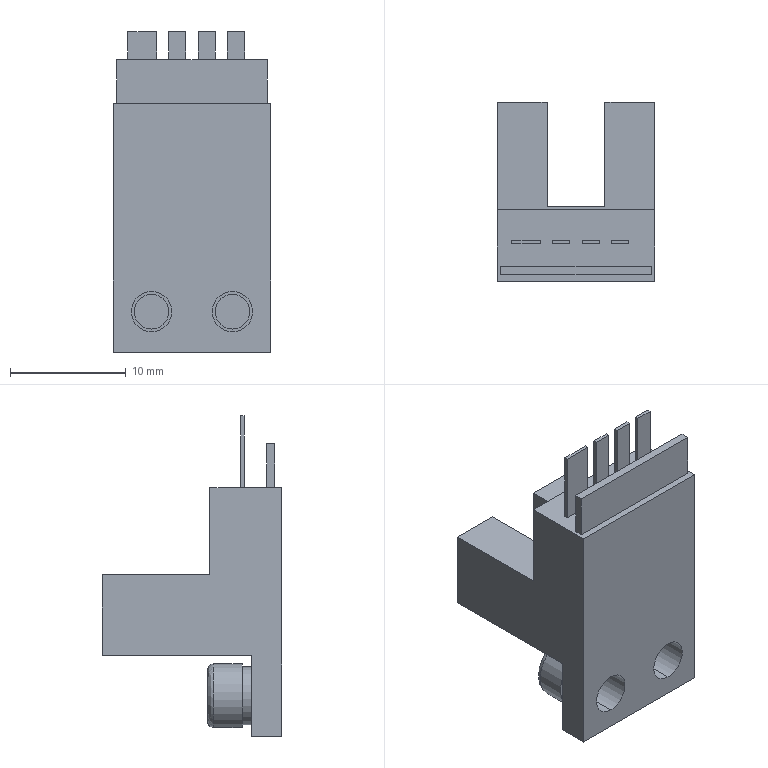Part | SolidWorks | features BaseBody 1 | 1 solid | 91 faces | box 13.6 x 15.5 x 27.7 mm | volume 2180 mm3 | plane 71 | cylinder 16 | spline 4 | commonest cylinder face diameters 3 x4 3.5 x4 5 x4 5.5 x4